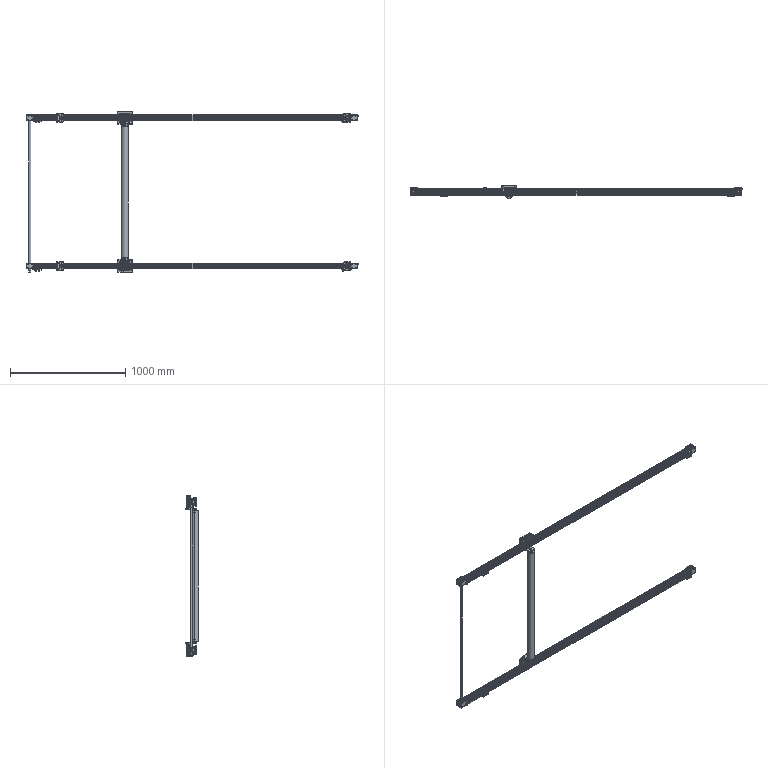Part | SolidWorks | features CompositeCurve 1, MirrorCompFeat 1, ReferencePattern 1 | 55 solids | 11360 faces | volume 15688667 mm3 | plane 6022 | cylinder 3362 | cone 1298 | spline 466 | torus 188 | sphere 24 | commonest cylinder face diameters 0.2 x764 2 x242 0.4 x238 5.5 x200 5 x154 10 x148